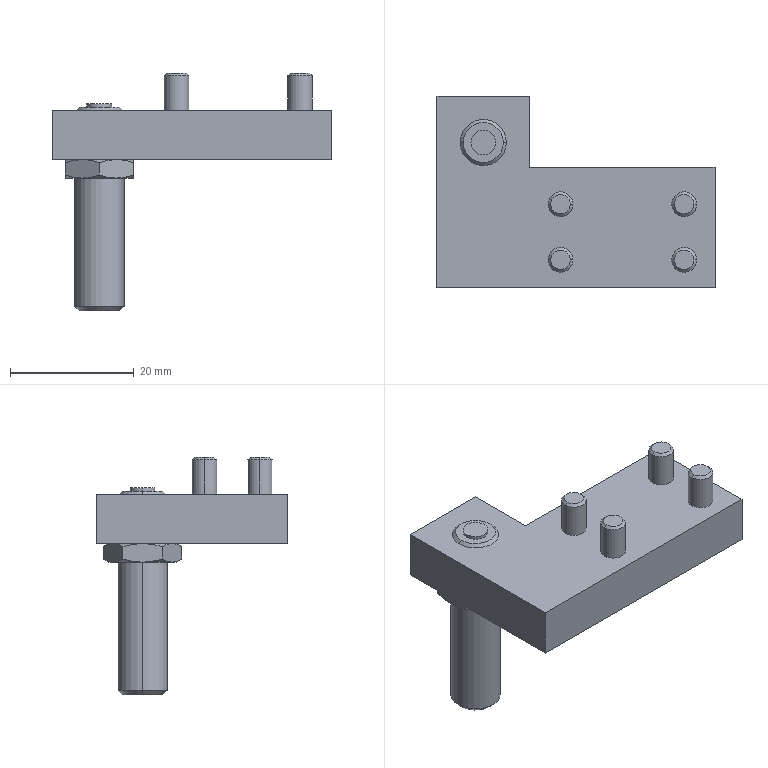Part | STEP file | QA-HI_MDX12_BB | 1 solid | 106 faces | box 45 x 31 x 38.5 mm | volume 10085 mm3 | plane 54 | cone 24 | cylinder 20 | spline 8 | commonest cylinder face diameters 4 x10 7.5 x8 8 x2